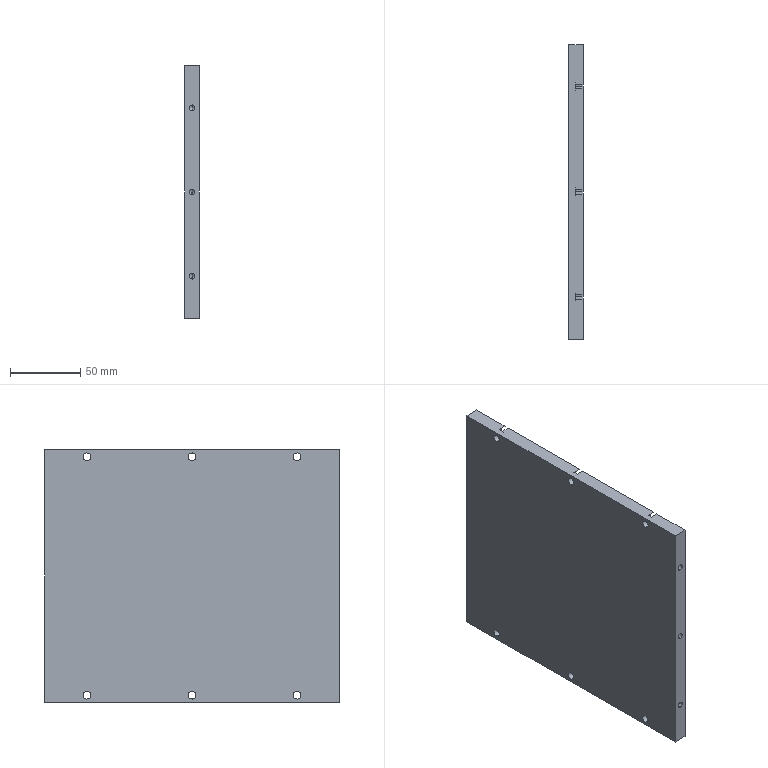Part | STEP file | 03-01 Loading-unloading side plate 1 | 1 solid | 45 faces | box 10 x 210 x 180 mm | volume 373986 mm3 | cylinder 27 | plane 12 | cone 6 | commonest cylinder face diameters 5.5 x12 10.5 x9 4.2 x6